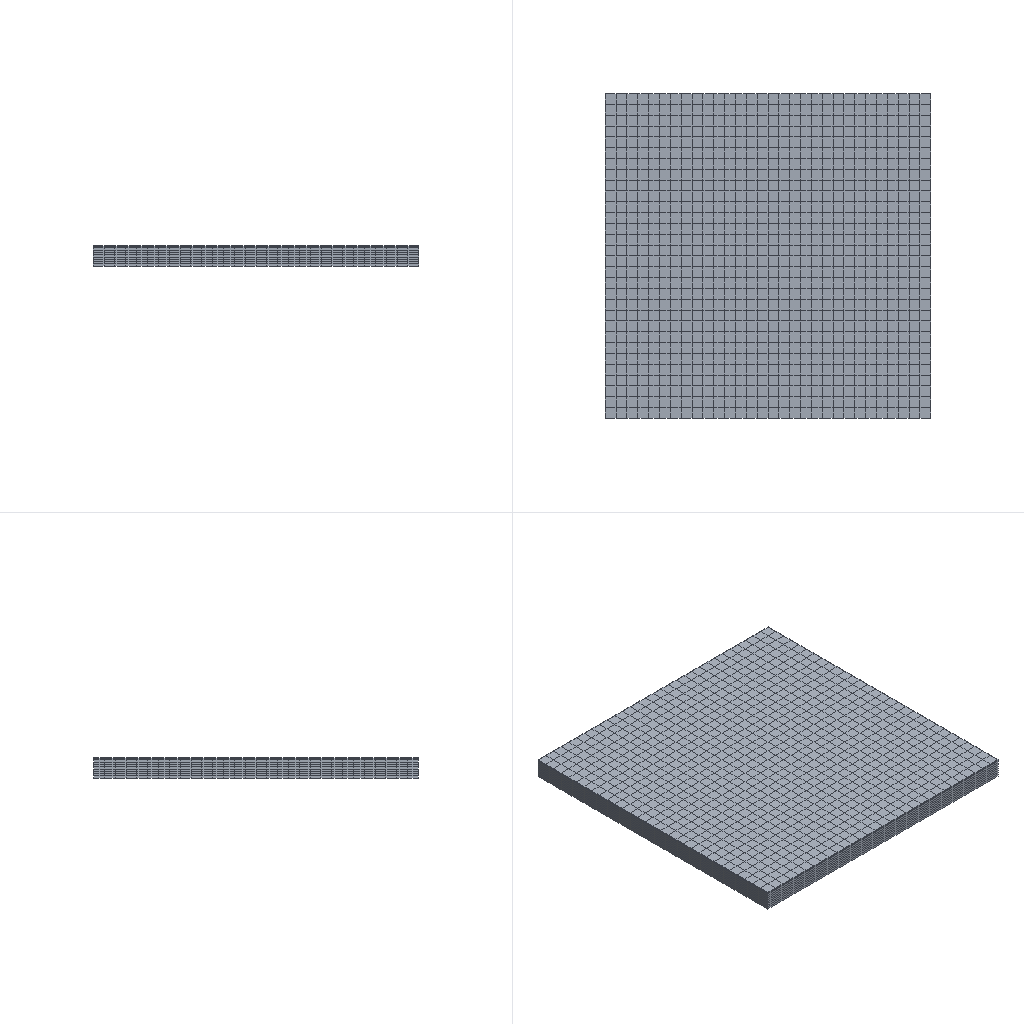Simulation study | abaqus
Set-up summary:
category,name,step,type,value,unit,region
solver,abaqus
solver,version,,,Abaqus/Standard 2020
units,not stated in the deck,,not stated
analysis,deck,,soils,soils
load_step,Step-1,Step-1,soils
load_step,requested,,,1
mesh,nodes,,,10571
mesh,elements,,,9000
element_type,C3D8RP,,solid,9000
load,load commands in deck,,count,1
bc,support commands in deck,,count,4
material,FENZHI,,in results
material,NIANTU,,in results
material,SHA,,in results
material,SUTIANTU,,in results
material,YUNI,,in results
check,setup vs results,,match,"per instance, exact: element labels, types and connectivity; labels of the nodes the elements use; coordinates of those nodes at SINGLE_PRECISION in 1 of 1 instance(s)"
Abaqus input file, long lists of numbers shortened:
*Heading
** Job name: Job-2 Model name: Model-1-Copy
** Generated by: Abaqus/CAE 2020
*Preprint, echo=NO, model=NO, history=NO, contact=NO
**
** PARTS
**
*Part, name=new
*Node
      1,           0.,           0.,    2.1
      2,           0.,  -148.9,    2.1
** (10569 more lines like these left out)
*Element, type=C3D8RP
   1,  206,  973, 6367,  857,    1,   25,  741,   86
   2,  973,  974, 6368, 6367,   25,   26,  742,  741
** (8998 more lines like these left out)
*Nset, nset=Set-1
   15,   16,   18,   19,   21,   22,   23,   24,  414,  415,  416,  417,  418,  419,  420,  421
  422,  423,  424,  425,  426,  427,  428,  429,  430,  431,  432,  433,  434,  435,  436,  437
** (119 more lines like these left out)
*Elset, elset=Set-1, generate
 8101,  9000,     1
*Nset, nset=Set-2
   13,   14,   15,   16,   17,   18,   19,   20,  385,  386,  387,  388,  389,  390,  391,  392
  393,  394,  395,  396,  397,  398,  399,  400,  401,  402,  403,  404,  405,  406,  407,  408
** (119 more lines like these left out)
*Elset, elset=Set-2, generate
 4501,  5400,     1
*Nset, nset=Set-3
     3,     4,     6,     7,    13,    14,    17,    20,    56,    57,    58,    59,    60,    61,    62,    63
    64,    65,    66,    67,    68,    69,    70,    71,    72,    73,    74,    75,    76,    77,    78,    79
** (239 more lines like these left out)
*Elset, elset=Set-3, generate
 5401,  8100,     1
*Nset, nset=Set-4
    1,    2,    3,    4,    5,    6,    7,    8,   25,   26,   27,   28,   29,   30,   31,   32
   33,   34,   35,   36,   37,   38,   39,   40,   41,   42,   43,   44,   45,   46,   47,   48
** (239 more lines like these left out)
*Elset, elset=Set-4, generate
    1,  2700,     1
*Nset, nset=Set-5
    1,    2,    5,    8,    9,   10,   11,   12,   25,   26,   27,   28,   29,   30,   31,   32
   33,   34,   35,   36,   37,   38,   39,   40,   41,   42,   43,   44,   45,   46,   47,   48
** (179 more lines like these left out)
*Elset, elset=Set-5, generate
 2701,  4500,     1
*Orientation, name=Ori-1
1., 0., 0., 0., 1., 0.
1, 0.
** Section: niantu
*Solid Section, elset=Set-4, orientation=Ori-1, material=niantu
,
** Section: fenzhi
*Solid Section, elset=Set-5, orientation=Ori-1, material=fenzhi
,
** Section: sutian
*Solid Section, elset=Set-2, orientation=Ori-1, material=sutiantu
,
** Section: yuni
*Solid Section, elset=Set-3, orientation=Ori-1, material=yuni
,
** Section: sha
*Solid Section, elset=Set-1, orientation=Ori-1, material=sha
,
*End Part
**
**
** ASSEMBLY
**
*Assembly, name=Assembly
**
*Instance, name=new-1, part=new
*End Instance
**
*Nset, nset=Set-11, instance=new-1
    1,    2,    3,    4,    5,    6,    7,    8,    9,   10,   11,   12,   13,   14,   15,   16
   17,   18,   19,   20,   21,   22,   23,   24,   54,   55,   85,   86,  116,  117,  147,  148
** (41 more lines like these left out)
*Elset, elset=Set-11, instance=new-1
    1,   30,   31,   60,   61,   90,   91,  120,  121,  150,  151,  180,  181,  210,  211,  240
  241,  270,  271,  300,  301,  330,  331,  360,  361,  390,  391,  420,  421,  450,  451,  480
** (36 more lines like these left out)
*Nset, nset=Set-12, instance=new-1
    1,    2,    3,    4,    5,    6,    7,    8,    9,   10,   11,   12,   13,   14,   15,   16
   17,   18,   19,   20,   21,   22,   23,   24,   25,   26,   27,   28,   29,   30,   31,   32
** (41 more lines like these left out)
*Elset, elset=Set-12, instance=new-1
    1,    2,    3,    4,    5,    6,    7,    8,    9,   10,   11,   12,   13,   14,   15,   16
   17,   18,   19,   20,   21,   22,   23,   24,   25,   26,   27,   28,   29,   30,   31,   32
** (36 more lines like these left out)
*Nset, nset=Set-13, instance=new-1
    9,   10,   11,   12,  266,  267,  268,  269,  270,  271,  272,  273,  274,  275,  276,  277
  278,  279,  280,  281,  282,  283,  284,  285,  286,  287,  288,  289,  290,  291,  292,  293
** (59 more lines like these left out)
*Elset, elset=Set-13, instance=new-1
 2731, 2732, 2733, 2734, 2735, 2736, 2737, 2738, 2739, 2740, 2741, 2742, 2743, 2744, 2745, 2746
 2747, 2748, 2749, 2750, 2751, 2752, 2753, 2754, 2755, 2756, 2757, 2758, 2759, 2760, 2791, 2792
** (55 more lines like these left out)
*Nset, nset=Set-14, instance=new-1
   21,   22,   23,   24,  625,  626,  627,  628,  629,  630,  631,  632,  633,  634,  635,  636
  637,  638,  639,  640,  641,  642,  643,  644,  645,  646,  647,  648,  649,  650,  651,  652
** (59 more lines like these left out)
*Elset, elset=Set-14, instance=new-1, generate
 8101,  9000,     1
*Nset, nset=Set-15, instance=new-1, generate
     1,  10571,      1
*Elset, elset=Set-15, instance=new-1, generate
    1,  9000,     1
*Nset, nset=Set-16, instance=new-1, generate
     1,  10571,      1
*Elset, elset=Set-16, instance=new-1, generate
    1,  9000,     1
*Nset, nset=Set-17, instance=new-1
   15,   16,   18,   19,   21,   22,   23,   24,  414,  415,  416,  417,  418,  419,  420,  421
  422,  423,  424,  425,  426,  427,  428,  429,  430,  431,  432,  433,  434,  435,  436,  437
** (119 more lines like these left out)
*Elset, elset=Set-17, instance=new-1, generate
 8101,  9000,     1
*Nset, nset=Set-18, instance=new-1
     1,     2,     3,     4,     5,     6,     7,     8,     9,    10,    11,    12,    13,    14,    15,    16
    17,    18,    19,    20,    25,    26,    27,    28,    29,    30,    31,    32,    33,    34,    35,    36
** (599 more lines like these left out)
*Elset, elset=Set-18, instance=new-1, generate
    1,  8100,     1
*Elset, elset=_Surf-2_S5, internal, instance=new-1, generate
 8101,  9000,     1
*Surface, type=ELEMENT, name=Surf-2
_Surf-2_S5, S5
*Nset, nset=Set-14_PP_, internal, instance=new-1
   21,   22,   23,   24,  625,  626,  627,  628,  629,  630,  631,  632,  633,  634,  635,  636
  637,  638,  639,  640,  641,  642,  643,  644,  645,  646,  647,  648,  649,  650,  651,  652
** (59 more lines like these left out)
*End Assembly
*Amplitude, name=Amp-1
             0.,              0.,              1.,              1.
**
** MATERIALS
**
*Material, name=fenzhi
*Elastic
 7.89e+06, 0.35
*Gap Flow
 0.001,
*Permeability, specific=9800., type=ORTHOTROPIC
 5.17e-07, 5.17e-07, 5.85e-07,   0.0105
*Mohr Coulomb
 11.6, 0.1
*Mohr Coulomb Hardening
31500.,0.
*Material, name=niantu
*Elastic
 6.95e+06, 0.4
*Gap Flow
 0.001,
*Permeability, specific=9800., type=ORTHOTROPIC
 5.05e-07, 5.05e-07, 5.52e-07,   0.0125
*Mohr Coulomb
 20.4, 0.1
*Mohr Coulomb Hardening
30000.,0.
*Material, name=sha
*Elastic
 1.37e+07, 0.32
*Gap Flow
 0.001,
*Permeability, specific=9800., type=ORTHOTROPIC
 2.5e-05, 2.5e-05, 2.5e-05,  0.0223
*Mohr Coulomb
23., 0.1
*Mohr Coulomb Hardening
 0.1,0.
*Material, name=sutiantu
*Elastic
 8.85e+06, 0.18
*Gap Flow
 0.001,
*Permeability, specific=9800., type=ORTHOTROPIC
 4.07e-07, 4.07e-07, 4.72e-07,   0.0068
*Mohr Coulomb
 23.1, 0.1
*Mohr Coulomb Hardening
42000.,0.
*Material, name=yuni
*Elastic
 2.86e+06, 0.3
*Gap Flow
 0.001,
*Permeability, specific=9800., type=ORTHOTROPIC
 4.01e-07, 4.01e-07, 4.42e-07,   0.0173
*Mohr Coulomb
 9.8, 0.1
*Mohr Coulomb Hardening
19800.,0.
**
** PREDEFINED FIELDS
**
** Name: Predefined Field-1   Type: Void ratio
*Initial Conditions, TYPE=RATIO
Set-15, 0.2
** Name: Predefined Field-2   Type: Pore pressure
*Initial Conditions, TYPE=PORE PRESSURE
Set-17, 500000.
** Name: Predefined Field-middle Type: [REDACTED] [REDACTED]
*Initial Conditions, TYPE=PORE PRESSURE
Set-18, 5e+09
** ----------------------------------------------------------------
**
** STEP: Step-1
**
*Step, name=Step-1, nlgeom=YES, inc=10000, unsymm=YES
*Soils, consolidation, end=PERIOD, utol=1e+19, stabilize=0.0002, allsdtol=0.05, continue=NO
1., 5.184e+06, 0.1, 5.184e+06,
**
** BOUNDARY CONDITIONS
**
** Name: BC-1 Type: 位移/转角
*Boundary
Set-11, 2, 2
** Name: BC-2 Type: 位移/转角
*Boundary
Set-12, 1, 1
** Name: BC-3 Type: 位移/转角
*Boundary
Set-13, 3, 3
** Name: [REDACTED] : Pore pressure
*Boundary
Set-14_PP_, 8, 8
**
** LOADS
**
** Name: Load-1   Type: Pressure
*Dsload, amplitude=Amp-1
Surf-2, P, 90000.
**
** OUTPUT REQUESTS
**
*Restart, write, frequency=0
**
** FIELD OUTPUT: F-Output-1
**
*Output, field
*Node Output
POR, RF, RT, U, V
*Element Output, directions=YES
E, FLUVR, FLVEL, LE, MISES, MISESMAX, PE, PEEQ, PEEQMAX, PEEQT, PEMAG, PEQC, S, SAT, VE, VEEQ
VOIDR
*Output, history, frequency=0
*End Step
Results summary:
result,step,,completed,increments=37 time=5184000.0/5184000.0
result,analysis,,,"soils, consolidation"
result,last_loadstep,,,1
result,primary field,,,"U, POR"
result,reaction total,,FX,0.0,model units
result,reaction total,,FY,0.0,model units
result,reaction total,,FZ,1999429075.688,model units